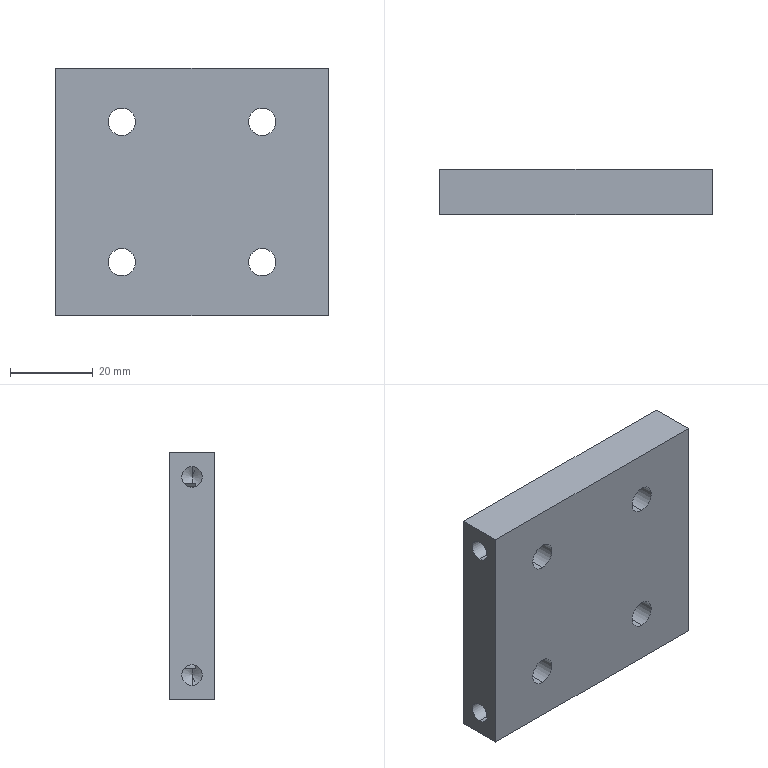Part | STEP file | 1 solid | 42 faces | box 66 x 11 x 60 mm | volume 39291 mm3 | cylinder 24 | plane 10 | cone 8 | commonest cylinder face diameters 5 x8 6.6 x8 11 x8